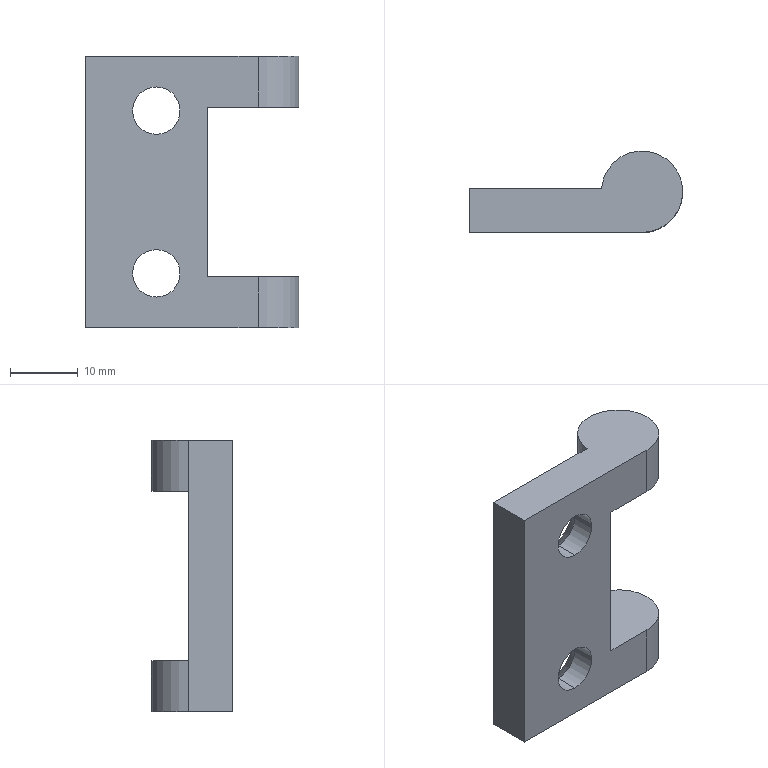Part | SolidWorks | features ICE 3, Chamfer 1, Extrusion 1 | 1 solid | 20 faces | box 31.5 x 12 x 40 mm | volume 5884 mm3 | cylinder 8 | plane 8 | cone 4 | commonest cylinder face diameters 7 x4 12 x4
STEP:
#1=CARTESIAN_POINT('',(-2.25,3.5,-15.5));
#2=VERTEX_POINT('',#1);
#3=CARTESIAN_POINT('',(-2.25,3.5,-8.5));
#4=VERTEX_POINT('',#3);
#5=CARTESIAN_POINT('',(-2.25,3.5,-12.));
#6=DIRECTION('',(0.,1.,0.));
#7=DIRECTION('',(0.,0.,1.));
#8=AXIS2_PLACEMENT_3D('',#5,#6,#7);
#9=CIRCLE('',#8,3.5);
#10=EDGE_CURVE('',#2,#4,#9,.T.);
#11=ORIENTED_EDGE('',*,*,#10,.F.);
#12=CARTESIAN_POINT('',(-2.25,6.5,-18.5));
#13=VERTEX_POINT('',#12);
#14=CARTESIAN_POINT('',(-2.25,3.5,-15.5));
#15=DIRECTION('',(0.,0.7071,-0.7071));
#16=VECTOR('',#15,1000.);
#17=LINE('',#14,#16);
#18=EDGE_CURVE('',#2,#13,#17,.T.);
#19=ORIENTED_EDGE('',*,*,#18,.T.);
#20=CARTESIAN_POINT('',(-2.25,6.5,-5.5));
#21=VERTEX_POINT('',#20);
#22=CARTESIAN_POINT('',(-2.25,6.5,-12.));
#23=DIRECTION('',(0.,-1.,0.));
#24=DIRECTION('',(0.,0.,1.));
#25=AXIS2_PLACEMENT_3D('',#22,#23,#24);
#26=CIRCLE('',#25,6.5);
#27=EDGE_CURVE('',#21,#13,#26,.T.);
#28=ORIENTED_EDGE('',*,*,#27,.F.);
#29=CARTESIAN_POINT('',(-2.25,3.5,-8.5));
#30=DIRECTION('',(0.,0.7071,0.7071));
#31=VECTOR('',#30,1000.);
#32=LINE('',#29,#31);
#33=EDGE_CURVE('',#4,#21,#32,.T.);
#34=ORIENTED_EDGE('',*,*,#33,.F.);
#35=EDGE_LOOP('',(#11,#19,#28,#34));
#36=FACE_OUTER_BOUND('',#35,.T.);
#37=CARTESIAN_POINT('',(-2.25,3.5,-12.));
#38=DIRECTION('',(0.,1.,0.));
#39=DIRECTION('',(0.,0.,1.));
#40=AXIS2_PLACEMENT_3D('',#37,#38,#39);
#41=CONICAL_SURFACE('',#40,3.5,0.7854);
#42=ADVANCED_FACE('',(#36),#41,.F.);
#43=CARTESIAN_POINT('',(-2.25,3.5,8.5));
#44=VERTEX_POINT('',#43);
#45=CARTESIAN_POINT('',(-2.25,3.5,15.5));
#46=VERTEX_POINT('',#45);
#47=CARTESIAN_POINT('',(-2.25,3.5,12.));
#48=DIRECTION('',(0.,1.,0.));
#49=DIRECTION('',(0.,0.,1.));
#50=AXIS2_PLACEMENT_3D('',#47,#48,#49);
#51=CIRCLE('',#50,3.5);
#52=EDGE_CURVE('',#44,#46,#51,.T.);
#53=ORIENTED_EDGE('',*,*,#52,.F.);
#54=CARTESIAN_POINT('',(-2.25,6.5,5.5));
#55=VERTEX_POINT('',#54);
#56=CARTESIAN_POINT('',(-2.25,3.5,8.5));
#57=DIRECTION('',(0.,0.7071,-0.7071));
#58=VECTOR('',#57,1000.);
#59=LINE('',#56,#58);
#60=EDGE_CURVE('',#44,#55,#59,.T.);
#61=ORIENTED_EDGE('',*,*,#60,.T.);
#62=CARTESIAN_POINT('',(-2.25,6.5,18.5));
#63=VERTEX_POINT('',#62);
#64=CARTESIAN_POINT('',(-2.25,6.5,12.));
#65=DIRECTION('',(0.,-1.,0.));
#66=DIRECTION('',(0.,0.,1.));
#67=AXIS2_PLACEMENT_3D('',#64,#65,#66);
#68=CIRCLE('',#67,6.5);
#69=EDGE_CURVE('',#63,#55,#68,.T.);
#70=ORIENTED_EDGE('',*,*,#69,.F.);
#71=CARTESIAN_POINT('',(-2.25,3.5,15.5));
#72=DIRECTION('',(0.,0.7071,0.7071));
#73=VECTOR('',#72,1000.);
#74=LINE('',#71,#73);
#75=EDGE_CURVE('',#46,#63,#74,.T.);
#76=ORIENTED_EDGE('',*,*,#75,.F.);
#77=EDGE_LOOP('',(#53,#61,#70,#76));
#78=FACE_OUTER_BOUND('',#77,.T.);
#79=CARTESIAN_POINT('',(-2.25,3.5,12.));
#80=DIRECTION('',(0.,1.,0.));
#81=DIRECTION('',(0.,0.,1.));
#82=AXIS2_PLACEMENT_3D('',#79,#80,#81);
#83=CONICAL_SURFACE('',#82,3.5,0.7854);
#84=ADVANCED_FACE('',(#78),#83,.F.);
#85=CARTESIAN_POINT('',(-2.25,0.,8.5));
#86=VERTEX_POINT('',#85);
#87=CARTESIAN_POINT('',(-2.25,0.,15.5));
#88=VERTEX_POINT('',#87);
#89=CARTESIAN_POINT('',(-2.25,0.,12.));
#90=DIRECTION('',(0.,1.,0.));
#91=DIRECTION('',(0.,0.,1.));
#92=AXIS2_PLACEMENT_3D('',#89,#90,#91);
#93=CIRCLE('',#92,3.5);
#94=EDGE_CURVE('',#86,#88,#93,.T.);
#95=ORIENTED_EDGE('',*,*,#94,.F.);
#96=CARTESIAN_POINT('',(-2.25,0.,8.5));
#97=DIRECTION('',(0.,1.,0.));
#98=VECTOR('',#97,1000.);
#99=LINE('',#96,#98);
#100=EDGE_CURVE('',#86,#44,#99,.T.);
#101=ORIENTED_EDGE('',*,*,#100,.T.);
#102=ORIENTED_EDGE('',*,*,#52,.T.);
#103=CARTESIAN_POINT('',(-2.25,0.,15.5));
#104=DIRECTION('',(0.,1.,0.));
#105=VECTOR('',#104,1000.);
#106=LINE('',#103,#105);
#107=EDGE_CURVE('',#88,#46,#106,.T.);
#108=ORIENTED_EDGE('',*,*,#107,.F.);
#109=EDGE_LOOP('',(#95,#101,#102,#108));
#110=FACE_OUTER_BOUND('',#109,.T.);
#111=CARTESIAN_POINT('',(-2.25,0.,12.));
#112=DIRECTION('',(0.,1.,0.));
#113=DIRECTION('',(0.,0.,1.));
#114=AXIS2_PLACEMENT_3D('',#111,#112,#113);
#115=CYLINDRICAL_SURFACE('',#114,3.5);
#116=ADVANCED_FACE('',(#110),#115,.F.);
#117=CARTESIAN_POINT('',(-2.25,0.,-15.5));
#118=VERTEX_POINT('',#117);
#119=CARTESIAN_POINT('',(-2.25,0.,-8.5));
#120=VERTEX_POINT('',#119);
#121=CARTESIAN_POINT('',(-2.25,0.,-12.));
#122=DIRECTION('',(0.,1.,0.));
#123=DIRECTION('',(0.,0.,1.));
#124=AXIS2_PLACEMENT_3D('',#121,#122,#123);
#125=CIRCLE('',#124,3.5);
#126=EDGE_CURVE('',#118,#120,#125,.T.);
#127=ORIENTED_EDGE('',*,*,#126,.F.);
#128=CARTESIAN_POINT('',(-2.25,0.,-15.5));
#129=DIRECTION('',(0.,1.,0.));
#130=VECTOR('',#129,1000.);
#131=LINE('',#128,#130);
#132=EDGE_CURVE('',#118,#2,#131,.T.);
#133=ORIENTED_EDGE('',*,*,#132,.T.);
#134=ORIENTED_EDGE('',*,*,#10,.T.);
#135=CARTESIAN_POINT('',(-2.25,0.,-8.5));
#136=DIRECTION('',(0.,1.,0.));
#137=VECTOR('',#136,1000.);
#138=LINE('',#135,#137);
#139=EDGE_CURVE('',#120,#4,#138,.T.);
#140=ORIENTED_EDGE('',*,*,#139,.F.);
#141=EDGE_LOOP('',(#127,#133,#134,#140));
#142=FACE_OUTER_BOUND('',#141,.T.);
#143=CARTESIAN_POINT('',(-2.25,0.,-12.));
#144=DIRECTION('',(0.,1.,0.));
#145=DIRECTION('',(0.,0.,1.));
#146=AXIS2_PLACEMENT_3D('',#143,#144,#145);
#147=CYLINDRICAL_SURFACE('',#146,3.5);
#148=ADVANCED_FACE('',(#142),#147,.F.);
#149=CARTESIAN_POINT('',(18.75,6.,12.5));
#150=VERTEX_POINT('',#149);
#151=CARTESIAN_POINT('',(12.75,0.,12.5));
#152=VERTEX_POINT('',#151);
#153=CARTESIAN_POINT('',(12.75,6.,12.5));
#154=DIRECTION('',(0.,0.,-1.));
#155=DIRECTION('',(1.,0.,0.));
#156=AXIS2_PLACEMENT_3D('',#153,#154,#155);
#157=CIRCLE('',#156,6.);
#158=EDGE_CURVE('',#150,#152,#157,.T.);
#159=ORIENTED_EDGE('',*,*,#158,.F.);
#160=CARTESIAN_POINT('',(18.75,6.,20.));
#161=VERTEX_POINT('',#160);
#162=CARTESIAN_POINT('',(18.75,6.,-36.971));
#163=DIRECTION('',(0.,0.,1.));
#164=VECTOR('',#163,1000.);
#165=LINE('',#162,#164);
#166=EDGE_CURVE('',#150,#161,#165,.T.);
#167=ORIENTED_EDGE('',*,*,#166,.T.);
#168=CARTESIAN_POINT('',(12.75,0.,20.));
#169=VERTEX_POINT('',#168);
#170=CARTESIAN_POINT('',(12.75,6.,20.));
#171=DIRECTION('',(0.,0.,1.));
#172=DIRECTION('',(1.,0.,0.));
#173=AXIS2_PLACEMENT_3D('',#170,#171,#172);
#174=CIRCLE('',#173,6.);
#175=EDGE_CURVE('',#169,#161,#174,.T.);
#176=ORIENTED_EDGE('',*,*,#175,.F.);
#177=CARTESIAN_POINT('',(12.75,0.,-20.));
#178=DIRECTION('',(0.,0.,-1.));
#179=VECTOR('',#178,1000.);
#180=LINE('',#177,#179);
#181=EDGE_CURVE('',#169,#152,#180,.T.);
#182=ORIENTED_EDGE('',*,*,#181,.T.);
#183=EDGE_LOOP('',(#159,#167,#176,#182));
#184=FACE_OUTER_BOUND('',#183,.T.);
#185=CARTESIAN_POINT('',(12.75,6.,-36.971));
#186=DIRECTION('',(0.,0.,1.));
#187=DIRECTION('',(1.,0.,0.));
#188=AXIS2_PLACEMENT_3D('',#185,#186,#187);
#189=CYLINDRICAL_SURFACE('',#188,6.);
#190=ADVANCED_FACE('',(#184),#189,.T.);
#191=CARTESIAN_POINT('',(18.75,6.,-20.));
#192=VERTEX_POINT('',#191);
#193=CARTESIAN_POINT('',(12.75,0.,-20.));
#194=VERTEX_POINT('',#193);
#195=CARTESIAN_POINT('',(12.75,6.,-20.));
#196=DIRECTION('',(0.,0.,-1.));
#197=DIRECTION('',(1.,0.,0.));
#198=AXIS2_PLACEMENT_3D('',#195,#196,#197);
#199=CIRCLE('',#198,6.);
#200=EDGE_CURVE('',#192,#194,#199,.T.);
#201=ORIENTED_EDGE('',*,*,#200,.F.);
#202=CARTESIAN_POINT('',(18.75,6.,-12.5));
#203=VERTEX_POINT('',#202);
#204=CARTESIAN_POINT('',(18.75,6.,-36.971));
#205=DIRECTION('',(0.,0.,1.));
#206=VECTOR('',#205,1000.);
#207=LINE('',#204,#206);
#208=EDGE_CURVE('',#192,#203,#207,.T.);
#209=ORIENTED_EDGE('',*,*,#208,.T.);
#210=CARTESIAN_POINT('',(12.75,0.,-12.5));
#211=VERTEX_POINT('',#210);
#212=CARTESIAN_POINT('',(12.75,6.,-12.5));
#213=DIRECTION('',(0.,0.,1.));
#214=DIRECTION('',(-1.,0.,0.));
#215=AXIS2_PLACEMENT_3D('',#212,#213,#214);
#216=CIRCLE('',#215,6.);
#217=EDGE_CURVE('',#211,#203,#216,.T.);
#218=ORIENTED_EDGE('',*,*,#217,.F.);
#219=CARTESIAN_POINT('',(12.75,0.,-20.));
#220=DIRECTION('',(0.,0.,-1.));
#221=VECTOR('',#220,1000.);
#222=LINE('',#219,#221);
#223=EDGE_CURVE('',#211,#194,#222,.T.);
#224=ORIENTED_EDGE('',*,*,#223,.T.);
#225=EDGE_LOOP('',(#201,#209,#218,#224));
#226=FACE_OUTER_BOUND('',#225,.T.);
#227=CARTESIAN_POINT('',(12.75,6.,-36.971));
#228=DIRECTION('',(0.,0.,1.));
#229=DIRECTION('',(1.,0.,0.));
#230=AXIS2_PLACEMENT_3D('',#227,#228,#229);
#231=CYLINDRICAL_SURFACE('',#230,6.);
#232=ADVANCED_FACE('',(#226),#231,.T.);
#233=ORIENTED_EDGE('',*,*,#208,.F.);
#234=CARTESIAN_POINT('',(6.771,6.5,-20.));
#235=VERTEX_POINT('',#234);
#236=CARTESIAN_POINT('',(12.75,6.,-20.));
#237=DIRECTION('',(0.,0.,-1.));
#238=DIRECTION('',(1.,0.,0.));
#239=AXIS2_PLACEMENT_3D('',#236,#237,#238);
#240=CIRCLE('',#239,6.);
#241=EDGE_CURVE('',#235,#192,#240,.T.);
#242=ORIENTED_EDGE('',*,*,#241,.F.);
#243=CARTESIAN_POINT('',(6.771,6.5,-12.5));
#244=VERTEX_POINT('',#243);
#245=CARTESIAN_POINT('',(6.771,6.5,-36.971));
#246=DIRECTION('',(0.,0.,1.));
#247=VECTOR('',#246,1000.);
#248=LINE('',#245,#247);
#249=EDGE_CURVE('',#235,#244,#248,.T.);
#250=ORIENTED_EDGE('',*,*,#249,.T.);
#251=CARTESIAN_POINT('',(12.75,6.,-12.5));
#252=DIRECTION('',(0.,0.,1.));
#253=DIRECTION('',(-1.,0.,0.));
#254=AXIS2_PLACEMENT_3D('',#251,#252,#253);
#255=CIRCLE('',#254,6.);
#256=EDGE_CURVE('',#203,#244,#255,.T.);
#257=ORIENTED_EDGE('',*,*,#256,.F.);
#258=EDGE_LOOP('',(#233,#242,#250,#257));
#259=FACE_OUTER_BOUND('',#258,.T.);
#260=CARTESIAN_POINT('',(12.75,6.,-36.971));
#261=DIRECTION('',(0.,0.,1.));
#262=DIRECTION('',(1.,0.,0.));
#263=AXIS2_PLACEMENT_3D('',#260,#261,#262);
#264=CYLINDRICAL_SURFACE('',#263,6.);
#265=ADVANCED_FACE('',(#259),#264,.T.);
#266=ORIENTED_EDGE('',*,*,#241,.T.);
#267=ORIENTED_EDGE('',*,*,#200,.T.);
#268=CARTESIAN_POINT('',(-12.75,0.,-20.));
#269=VERTEX_POINT('',#268);
#270=CARTESIAN_POINT('',(-12.75,0.,-20.));
#271=DIRECTION('',(-1.,0.,0.));
#272=VECTOR('',#271,1000.);
#273=LINE('',#270,#272);
#274=EDGE_CURVE('',#194,#269,#273,.T.);
#275=ORIENTED_EDGE('',*,*,#274,.T.);
#276=CARTESIAN_POINT('',(-12.75,6.5,-20.));
#277=VERTEX_POINT('',#276);
#278=CARTESIAN_POINT('',(-12.75,6.5,-20.));
#279=DIRECTION('',(0.,-1.,0.));
#280=VECTOR('',#279,1000.);
#281=LINE('',#278,#280);
#282=EDGE_CURVE('',#277,#269,#281,.T.);
#283=ORIENTED_EDGE('',*,*,#282,.F.);
#284=CARTESIAN_POINT('',(-12.75,6.5,-20.));
#285=DIRECTION('',(-1.,0.,0.));
#286=VECTOR('',#285,1000.);
#287=LINE('',#284,#286);
#288=EDGE_CURVE('',#235,#277,#287,.T.);
#289=ORIENTED_EDGE('',*,*,#288,.F.);
#290=EDGE_LOOP('',(#266,#267,#275,#283,#289));
#291=FACE_OUTER_BOUND('',#290,.T.);
#292=CARTESIAN_POINT('',(-12.75,6.5,-20.));
#293=DIRECTION('',(0.,0.,1.));
#294=DIRECTION('',(1.,0.,0.));
#295=AXIS2_PLACEMENT_3D('',#292,#293,#294);
#296=PLANE('',#295);
#297=ADVANCED_FACE('',(#291),#296,.F.);
#298=CARTESIAN_POINT('',(-12.75,0.,20.));
#299=VERTEX_POINT('',#298);
#300=CARTESIAN_POINT('',(-12.75,0.,-20.));
#301=DIRECTION('',(0.,0.,1.));
#302=VECTOR('',#301,1000.);
#303=LINE('',#300,#302);
#304=EDGE_CURVE('',#269,#299,#303,.T.);
#305=ORIENTED_EDGE('',*,*,#304,.T.);
#306=CARTESIAN_POINT('',(-12.75,6.5,20.));
#307=VERTEX_POINT('',#306);
#308=CARTESIAN_POINT('',(-12.75,6.5,20.));
#309=DIRECTION('',(0.,-1.,0.));
#310=VECTOR('',#309,1000.);
#311=LINE('',#308,#310);
#312=EDGE_CURVE('',#307,#299,#311,.T.);
#313=ORIENTED_EDGE('',*,*,#312,.F.);
#314=CARTESIAN_POINT('',(-12.75,6.5,-20.));
#315=DIRECTION('',(0.,0.,1.));
#316=VECTOR('',#315,1000.);
#317=LINE('',#314,#316);
#318=EDGE_CURVE('',#277,#307,#317,.T.);
#319=ORIENTED_EDGE('',*,*,#318,.F.);
#320=ORIENTED_EDGE('',*,*,#282,.T.);
#321=EDGE_LOOP('',(#305,#313,#319,#320));
#322=FACE_OUTER_BOUND('',#321,.T.);
#323=CARTESIAN_POINT('',(-12.75,6.5,-20.));
#324=DIRECTION('',(1.,0.,0.));
#325=DIRECTION('',(0.,0.,-1.));
#326=AXIS2_PLACEMENT_3D('',#323,#324,#325);
#327=PLANE('',#326);
#328=ADVANCED_FACE('',(#322),#327,.F.);
#329=CARTESIAN_POINT('',(-12.75,0.,20.));
#330=DIRECTION('',(1.,0.,0.));
#331=VECTOR('',#330,1000.);
#332=LINE('',#329,#331);
#333=EDGE_CURVE('',#299,#169,#332,.T.);
#334=ORIENTED_EDGE('',*,*,#333,.T.);
#335=ORIENTED_EDGE('',*,*,#175,.T.);
#336=CARTESIAN_POINT('',(6.771,6.5,20.));
#337=VERTEX_POINT('',#336);
#338=CARTESIAN_POINT('',(12.75,6.,20.));
#339=DIRECTION('',(0.,0.,1.));
#340=DIRECTION('',(1.,0.,0.));
#341=AXIS2_PLACEMENT_3D('',#338,#339,#340);
#342=CIRCLE('',#341,6.);
#343=EDGE_CURVE('',#161,#337,#342,.T.);
#344=ORIENTED_EDGE('',*,*,#343,.T.);
#345=CARTESIAN_POINT('',(-12.75,6.5,20.));
#346=DIRECTION('',(1.,0.,0.));
#347=VECTOR('',#346,1000.);
#348=LINE('',#345,#347);
#349=EDGE_CURVE('',#307,#337,#348,.T.);
#350=ORIENTED_EDGE('',*,*,#349,.F.);
#351=ORIENTED_EDGE('',*,*,#312,.T.);
#352=EDGE_LOOP('',(#334,#335,#344,#350,#351));
#353=FACE_OUTER_BOUND('',#352,.T.);
#354=CARTESIAN_POINT('',(-12.75,6.5,20.));
#355=DIRECTION('',(0.,0.,-1.));
#356=DIRECTION('',(-1.,0.,0.));
#357=AXIS2_PLACEMENT_3D('',#354,#355,#356);
#358=PLANE('',#357);
#359=ADVANCED_FACE('',(#353),#358,.F.);
#360=ORIENTED_EDGE('',*,*,#69,.T.);
#361=CARTESIAN_POINT('',(-2.25,6.5,12.));
#362=DIRECTION('',(0.,-1.,0.));
#363=DIRECTION('',(0.,0.,1.));
#364=AXIS2_PLACEMENT_3D('',#361,#362,#363);
#365=CIRCLE('',#364,6.5);
#366=EDGE_CURVE('',#55,#63,#365,.T.);
#367=ORIENTED_EDGE('',*,*,#366,.T.);
#368=EDGE_LOOP('',(#360,#367));
#369=FACE_BOUND('',#368,.T.);
#370=ORIENTED_EDGE('',*,*,#27,.T.);
#371=CARTESIAN_POINT('',(-2.25,6.5,-12.));
#372=DIRECTION('',(0.,-1.,0.));
#373=DIRECTION('',(0.,0.,1.));
#374=AXIS2_PLACEMENT_3D('',#371,#372,#373);
#375=CIRCLE('',#374,6.5);
#376=EDGE_CURVE('',#13,#21,#375,.T.);
#377=ORIENTED_EDGE('',*,*,#376,.T.);
#378=EDGE_LOOP('',(#370,#377));
#379=FACE_BOUND('',#378,.T.);
#380=CARTESIAN_POINT('',(5.25,6.5,12.5));
#381=VERTEX_POINT('',#380);
#382=CARTESIAN_POINT('',(6.771,6.5,12.5));
#383=VERTEX_POINT('',#382);
#384=CARTESIAN_POINT('',(0.,6.5,12.5));
#385=DIRECTION('',(1.,0.,0.));
#386=VECTOR('',#385,1000.);
#387=LINE('',#384,#386);
#388=EDGE_CURVE('',#381,#383,#387,.T.);
#389=ORIENTED_EDGE('',*,*,#388,.F.);
#390=CARTESIAN_POINT('',(5.25,6.5,-12.5));
#391=VERTEX_POINT('',#390);
#392=CARTESIAN_POINT('',(5.25,6.5,0.));
#393=DIRECTION('',(0.,0.,1.));
#394=VECTOR('',#393,1000.);
#395=LINE('',#392,#394);
#396=EDGE_CURVE('',#391,#381,#395,.T.);
#397=ORIENTED_EDGE('',*,*,#396,.F.);
#398=CARTESIAN_POINT('',(0.,6.5,-12.5));
#399=DIRECTION('',(-1.,0.,0.));
#400=VECTOR('',#399,1000.);
#401=LINE('',#398,#400);
#402=EDGE_CURVE('',#244,#391,#401,.T.);
#403=ORIENTED_EDGE('',*,*,#402,.F.);
#404=ORIENTED_EDGE('',*,*,#249,.F.);
#405=ORIENTED_EDGE('',*,*,#288,.T.);
#406=ORIENTED_EDGE('',*,*,#318,.T.);
#407=ORIENTED_EDGE('',*,*,#349,.T.);
#408=CARTESIAN_POINT('',(6.771,6.5,-36.971));
#409=DIRECTION('',(0.,0.,1.));
#410=VECTOR('',#409,1000.);
#411=LINE('',#408,#410);
#412=EDGE_CURVE('',#383,#337,#411,.T.);
#413=ORIENTED_EDGE('',*,*,#412,.F.);
#414=EDGE_LOOP('',(#389,#397,#403,#404,#405,#406,#407,#413));
#415=FACE_OUTER_BOUND('',#414,.T.);
#416=CARTESIAN_POINT('',(0.,6.5,0.));
#417=DIRECTION('',(0.,1.,0.));
#418=DIRECTION('',(0.,0.,1.));
#419=AXIS2_PLACEMENT_3D('',#416,#417,#418);
#420=PLANE('',#419);
#421=ADVANCED_FACE('',(#369,#379,#415),#420,.T.);
#422=CARTESIAN_POINT('',(-2.25,0.,12.));
#423=DIRECTION('',(0.,1.,0.));
#424=DIRECTION('',(0.,0.,1.));
#425=AXIS2_PLACEMENT_3D('',#422,#423,#424);
#426=CIRCLE('',#425,3.5);
#427=EDGE_CURVE('',#88,#86,#426,.T.);
#428=ORIENTED_EDGE('',*,*,#427,.T.);
#429=ORIENTED_EDGE('',*,*,#94,.T.);
#430=EDGE_LOOP('',(#428,#429));
#431=FACE_BOUND('',#430,.T.);
#432=CARTESIAN_POINT('',(-2.25,0.,-12.));
#433=DIRECTION('',(0.,1.,0.));
#434=DIRECTION('',(0.,0.,1.));
#435=AXIS2_PLACEMENT_3D('',#432,#433,#434);
#436=CIRCLE('',#435,3.5);
#437=EDGE_CURVE('',#120,#118,#436,.T.);
#438=ORIENTED_EDGE('',*,*,#437,.T.);
#439=ORIENTED_EDGE('',*,*,#126,.T.);
#440=EDGE_LOOP('',(#438,#439));
#441=FACE_BOUND('',#440,.T.);
#442=CARTESIAN_POINT('',(5.25,0.,12.5));
#443=VERTEX_POINT('',#442);
#444=CARTESIAN_POINT('',(5.25,0.,-12.5));
#445=VERTEX_POINT('',#444);
#446=CARTESIAN_POINT('',(5.25,0.,-12.5));
#447=DIRECTION('',(0.,0.,-1.));
#448=VECTOR('',#447,1000.);
#449=LINE('',#446,#448);
#450=EDGE_CURVE('',#443,#445,#449,.T.);
#451=ORIENTED_EDGE('',*,*,#450,.F.);
#452=CARTESIAN_POINT('',(32.25,0.,12.5));
#453=DIRECTION('',(-1.,0.,0.));
#454=VECTOR('',#453,1000.);
#455=LINE('',#452,#454);
#456=EDGE_CURVE('',#152,#443,#455,.T.);
#457=ORIENTED_EDGE('',*,*,#456,.F.);
#458=ORIENTED_EDGE('',*,*,#181,.F.);
#459=ORIENTED_EDGE('',*,*,#333,.F.);
#460=ORIENTED_EDGE('',*,*,#304,.F.);
#461=ORIENTED_EDGE('',*,*,#274,.F.);
#462=ORIENTED_EDGE('',*,*,#223,.F.);
#463=CARTESIAN_POINT('',(32.25,0.,-12.5));
#464=DIRECTION('',(1.,0.,0.));
#465=VECTOR('',#464,1000.);
#466=LINE('',#463,#465);
#467=EDGE_CURVE('',#445,#211,#466,.T.);
#468=ORIENTED_EDGE('',*,*,#467,.F.);
#469=EDGE_LOOP('',(#451,#457,#458,#459,#460,#461,#462,#468));
#470=FACE_OUTER_BOUND('',#469,.T.);
#471=CARTESIAN_POINT('',(0.,0.,0.));
#472=DIRECTION('',(0.,1.,0.));
#473=DIRECTION('',(0.,0.,1.));
#474=AXIS2_PLACEMENT_3D('',#471,#472,#473);
#475=PLANE('',#474);
#476=ADVANCED_FACE('',(#431,#441,#470),#475,.F.);
#477=ORIENTED_EDGE('',*,*,#166,.F.);
#478=CARTESIAN_POINT('',(12.75,6.,12.5));
#479=DIRECTION('',(0.,0.,-1.));
#480=DIRECTION('',(1.,0.,0.));
#481=AXIS2_PLACEMENT_3D('',#478,#479,#480);
#482=CIRCLE('',#481,6.);
#483=EDGE_CURVE('',#383,#150,#482,.T.);
#484=ORIENTED_EDGE('',*,*,#483,.F.);
#485=ORIENTED_EDGE('',*,*,#412,.T.);
#486=ORIENTED_EDGE('',*,*,#343,.F.);
#487=EDGE_LOOP('',(#477,#484,#485,#486));
#488=FACE_OUTER_BOUND('',#487,.T.);
#489=CARTESIAN_POINT('',(12.75,6.,-36.971));
#490=DIRECTION('',(0.,0.,1.));
#491=DIRECTION('',(1.,0.,0.));
#492=AXIS2_PLACEMENT_3D('',#489,#490,#491);
#493=CYLINDRICAL_SURFACE('',#492,6.);
#494=ADVANCED_FACE('',(#488),#493,.T.);
#495=ORIENTED_EDGE('',*,*,#396,.T.);
#496=CARTESIAN_POINT('',(5.25,12.,12.5));
#497=DIRECTION('',(0.,-1.,0.));
#498=VECTOR('',#497,1000.);
#499=LINE('',#496,#498);
#500=EDGE_CURVE('',#381,#443,#499,.T.);
#501=ORIENTED_EDGE('',*,*,#500,.T.);
#502=ORIENTED_EDGE('',*,*,#450,.T.);
#503=CARTESIAN_POINT('',(5.25,12.,-12.5));
#504=DIRECTION('',(0.,-1.,0.));
#505=VECTOR('',#504,1000.);
#506=LINE('',#503,#505);
#507=EDGE_CURVE('',#391,#445,#506,.T.);
#508=ORIENTED_EDGE('',*,*,#507,.F.);
#509=EDGE_LOOP('',(#495,#501,#502,#508));
#510=FACE_OUTER_BOUND('',#509,.T.);
#511=CARTESIAN_POINT('',(5.25,12.,-12.5));
#512=DIRECTION('',(-1.,0.,0.));
#513=DIRECTION('',(0.,0.,1.));
#514=AXIS2_PLACEMENT_3D('',#511,#512,#513);
#515=PLANE('',#514);
#516=ADVANCED_FACE('',(#510),#515,.F.);
#517=ORIENTED_EDGE('',*,*,#388,.T.);
#518=ORIENTED_EDGE('',*,*,#483,.T.);
#519=ORIENTED_EDGE('',*,*,#158,.T.);
#520=ORIENTED_EDGE('',*,*,#456,.T.);
#521=ORIENTED_EDGE('',*,*,#500,.F.);
#522=EDGE_LOOP('',(#517,#518,#519,#520,#521));
#523=FACE_OUTER_BOUND('',#522,.T.);
#524=CARTESIAN_POINT('',(32.25,12.,12.5));
#525=DIRECTION('',(0.,0.,1.));
#526=DIRECTION('',(1.,0.,0.));
#527=AXIS2_PLACEMENT_3D('',#524,#525,#526);
#528=PLANE('',#527);
#529=ADVANCED_FACE('',(#523),#528,.F.);
#530=ORIENTED_EDGE('',*,*,#402,.T.);
#531=ORIENTED_EDGE('',*,*,#507,.T.);
#532=ORIENTED_EDGE('',*,*,#467,.T.);
#533=ORIENTED_EDGE('',*,*,#217,.T.);
#534=ORIENTED_EDGE('',*,*,#256,.T.);
#535=EDGE_LOOP('',(#530,#531,#532,#533,#534));
#536=FACE_OUTER_BOUND('',#535,.T.);
#537=CARTESIAN_POINT('',(32.25,12.,-12.5));
#538=DIRECTION('',(0.,0.,-1.));
#539=DIRECTION('',(-1.,0.,0.));
#540=AXIS2_PLACEMENT_3D('',#537,#538,#539);
#541=PLANE('',#540);
#542=ADVANCED_FACE('',(#536),#541,.F.);
#543=ORIENTED_EDGE('',*,*,#132,.F.);
#544=ORIENTED_EDGE('',*,*,#437,.F.);
#545=ORIENTED_EDGE('',*,*,#139,.T.);
#546=CARTESIAN_POINT('',(-2.25,3.5,-12.));
#547=DIRECTION('',(0.,1.,0.));
#548=DIRECTION('',(0.,0.,1.));
#549=AXIS2_PLACEMENT_3D('',#546,#547,#548);
#550=CIRCLE('',#549,3.5);
#551=EDGE_CURVE('',#4,#2,#550,.T.);
#552=ORIENTED_EDGE('',*,*,#551,.T.);
#553=EDGE_LOOP('',(#543,#544,#545,#552));
#554=FACE_OUTER_BOUND('',#553,.T.);
#555=CARTESIAN_POINT('',(-2.25,0.,-12.));
#556=DIRECTION('',(0.,1.,0.));
#557=DIRECTION('',(0.,0.,1.));
#558=AXIS2_PLACEMENT_3D('',#555,#556,#557);
#559=CYLINDRICAL_SURFACE('',#558,3.5);
#560=ADVANCED_FACE('',(#554),#559,.F.);
#561=ORIENTED_EDGE('',*,*,#100,.F.);
#562=ORIENTED_EDGE('',*,*,#427,.F.);
#563=ORIENTED_EDGE('',*,*,#107,.T.);
#564=CARTESIAN_POINT('',(-2.25,3.5,12.));
#565=DIRECTION('',(0.,1.,0.));
#566=DIRECTION('',(0.,0.,1.));
#567=AXIS2_PLACEMENT_3D('',#564,#565,#566);
#568=CIRCLE('',#567,3.5);
#569=EDGE_CURVE('',#46,#44,#568,.T.);
#570=ORIENTED_EDGE('',*,*,#569,.T.);
#571=EDGE_LOOP('',(#561,#562,#563,#570));
#572=FACE_OUTER_BOUND('',#571,.T.);
#573=CARTESIAN_POINT('',(-2.25,0.,12.));
#574=DIRECTION('',(0.,1.,0.));
#575=DIRECTION('',(0.,0.,1.));
#576=AXIS2_PLACEMENT_3D('',#573,#574,#575);
#577=CYLINDRICAL_SURFACE('',#576,3.5);
#578=ADVANCED_FACE('',(#572),#577,.F.);
#579=ORIENTED_EDGE('',*,*,#60,.F.);
#580=ORIENTED_EDGE('',*,*,#569,.F.);
#581=ORIENTED_EDGE('',*,*,#75,.T.);
#582=ORIENTED_EDGE('',*,*,#366,.F.);
#583=EDGE_LOOP('',(#579,#580,#581,#582));
#584=FACE_OUTER_BOUND('',#583,.T.);
#585=CARTESIAN_POINT('',(-2.25,3.5,12.));
#586=DIRECTION('',(0.,1.,0.));
#587=DIRECTION('',(0.,0.,1.));
#588=AXIS2_PLACEMENT_3D('',#585,#586,#587);
#589=CONICAL_SURFACE('',#588,3.5,0.7854);
#590=ADVANCED_FACE('',(#584),#589,.F.);
#591=ORIENTED_EDGE('',*,*,#18,.F.);
#592=ORIENTED_EDGE('',*,*,#551,.F.);
#593=ORIENTED_EDGE('',*,*,#33,.T.);
#594=ORIENTED_EDGE('',*,*,#376,.F.);
#595=EDGE_LOOP('',(#591,#592,#593,#594));
#596=FACE_OUTER_BOUND('',#595,.T.);
#597=CARTESIAN_POINT('',(-2.25,3.5,-12.));
#598=DIRECTION('',(0.,1.,0.));
#599=DIRECTION('',(0.,0.,1.));
#600=AXIS2_PLACEMENT_3D('',#597,#598,#599);
#601=CONICAL_SURFACE('',#600,3.5,0.7854);
#602=ADVANCED_FACE('',(#596),#601,.F.);
#603=CLOSED_SHELL('',(#42,#84,#116,#148,#190,#232,#265,#297,#328,#359,#421,#476,#494,#516,#529,#542,#560,#578,#590,#602));
#604=MANIFOLD_SOLID_BREP('',#603);
#605=CARTESIAN_POINT('',(0.,0.,0.));
#606=DIRECTION('',(0.,0.,1.));
#607=DIRECTION('',(1.,0.,0.));
#608=AXIS2_PLACEMENT_3D('',#605,#606,#607);
#609=(LENGTH_UNIT()NAMED_UNIT(*)SI_UNIT(.MILLI.,.METRE.));
#610=UNCERTAINTY_MEASURE_WITH_UNIT(LENGTH_MEASURE(0.00001),#609,'','');
#611=(NAMED_UNIT(*)PLANE_ANGLE_UNIT()SI_UNIT($,.RADIAN.));
#612=(NAMED_UNIT(*)SI_UNIT($,.STERADIAN.)SOLID_ANGLE_UNIT());
#613=(GEOMETRIC_REPRESENTATION_CONTEXT(3)GLOBAL_UNCERTAINTY_ASSIGNED_CONTEXT((#610))GLOBAL_UNIT_ASSIGNED_CONTEXT((#609,#611,#612))REPRESENTATION_CONTEXT('',''));
#614=ADVANCED_BREP_SHAPE_REPRESENTATION('',(#604,#608),#613);